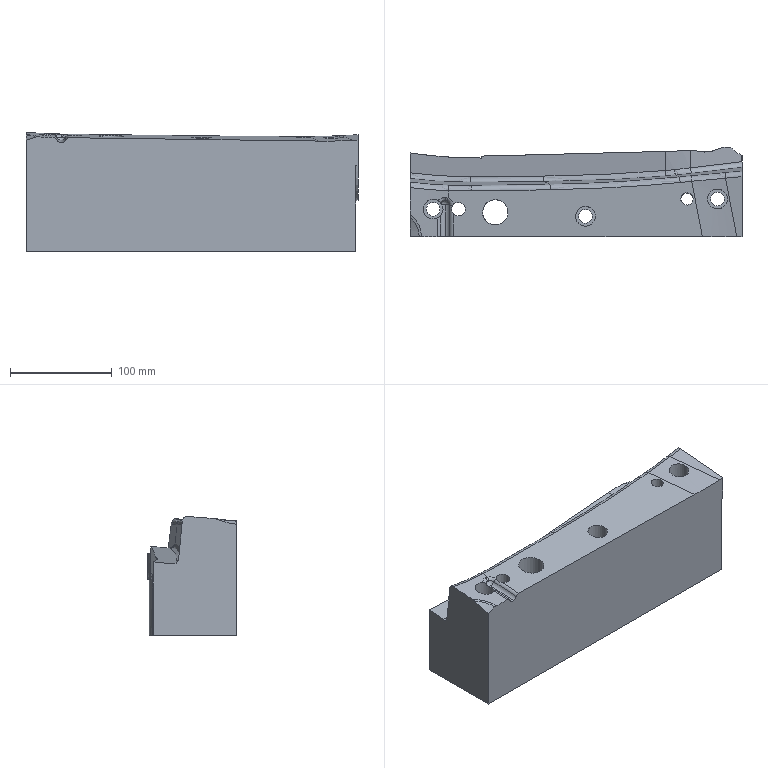Part | NX | features solid 2 | 1 solid | 63 faces | box 328.507 x 88.07 x 117.271 mm | volume 2538827 mm3 | spline 23 | cylinder 22 | plane 15 | cone 1 | sphere 1 | torus 1 | commonest cylinder face diameters 10 x6 13.5 x4 19.5 x3 7.999 x1 8 x1 9.999 x1